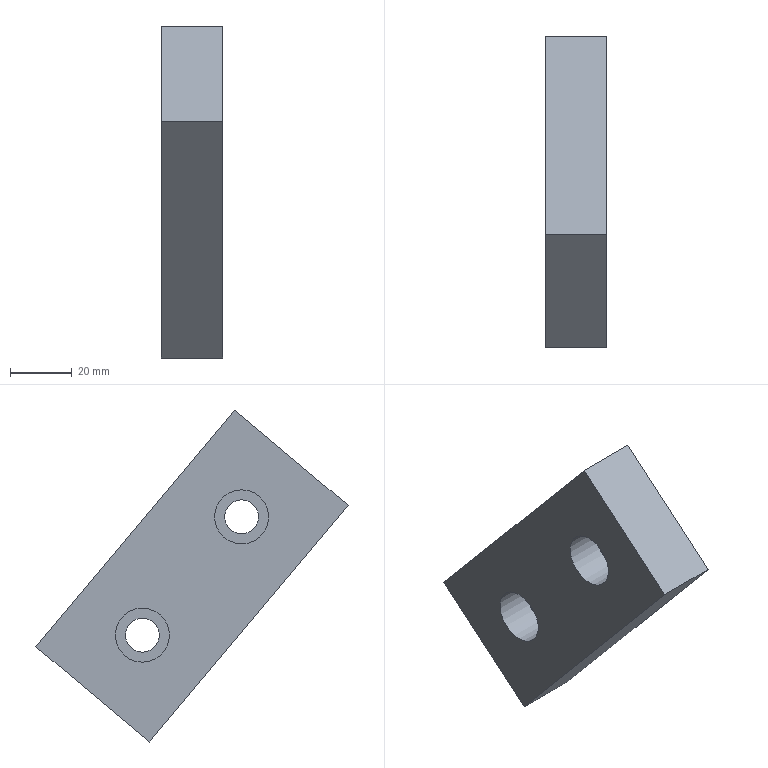Part | NX | features solid 2 | 1 solid | 12 faces | box 20 x 101.049 x 107.458 mm | volume 88707 mm3 | plane 8 | cylinder 4 | commonest cylinder face diameters 11 x2 17.5 x2
STEP:
#1=CARTESIAN_POINT('',(-585.,640.792,26.298));
#2=VERTEX_POINT('',#1);
#3=CARTESIAN_POINT('',(-585.,640.792,17.548));
#4=DIRECTION('',(-1.,0.,0.));
#5=DIRECTION('',(0.,0.,1.));
#6=AXIS2_PLACEMENT_3D('',#3,#4,#5);
#7=CIRCLE('',#6,8.75);
#8=EDGE_CURVE('',#2,#2,#7,.T.);
#9=ORIENTED_EDGE('',*,*,#8,.F.);
#10=EDGE_LOOP('',(#9));
#11=FACE_BOUND('',#10,.T.);
#12=CARTESIAN_POINT('',(-585.,608.652,64.601));
#13=VERTEX_POINT('',#12);
#14=CARTESIAN_POINT('',(-585.,608.652,55.851));
#15=DIRECTION('',(-1.,0.,0.));
#16=DIRECTION('',(0.,0.,1.));
#17=AXIS2_PLACEMENT_3D('',#14,#15,#16);
#18=CIRCLE('',#17,8.75);
#19=EDGE_CURVE('',#13,#13,#18,.T.);
#20=ORIENTED_EDGE('',*,*,#19,.F.);
#21=EDGE_LOOP('',(#20));
#22=FACE_BOUND('',#21,.T.);
#23=CARTESIAN_POINT('',(-585.,610.968,90.429));
#24=VERTEX_POINT('',#23);
#25=CARTESIAN_POINT('',(-585.,574.197,59.575));
#26=VERTEX_POINT('',#25);
#27=CARTESIAN_POINT('',(-585.,612.226,91.485));
#28=DIRECTION('',(0.,0.766,0.6428));
#29=VECTOR('',#28,1000.);
#30=LINE('',#27,#29);
#31=EDGE_CURVE('',#24,#26,#30,.F.);
#32=ORIENTED_EDGE('',*,*,#31,.F.);
#33=CARTESIAN_POINT('',(-585.,675.246,13.824));
#34=VERTEX_POINT('',#33);
#35=CARTESIAN_POINT('',(-585.,675.246,13.824));
#36=DIRECTION('',(0.,-0.6428,0.766));
#37=VECTOR('',#36,1000.);
#38=LINE('',#35,#37);
#39=EDGE_CURVE('',#34,#24,#38,.T.);
#40=ORIENTED_EDGE('',*,*,#39,.F.);
#41=CARTESIAN_POINT('',(-585.,638.476,-17.03));
#42=VERTEX_POINT('',#41);
#43=CARTESIAN_POINT('',(-585.,676.505,14.88));
#44=DIRECTION('',(0.,0.766,0.6428));
#45=VECTOR('',#44,1000.);
#46=LINE('',#43,#45);
#47=EDGE_CURVE('',#34,#42,#46,.F.);
#48=ORIENTED_EDGE('',*,*,#47,.T.);
#49=CARTESIAN_POINT('',(-585.,638.476,-17.03));
#50=DIRECTION('',(0.,0.6428,-0.766));
#51=VECTOR('',#50,1000.);
#52=LINE('',#49,#51);
#53=EDGE_CURVE('',#42,#26,#52,.F.);
#54=ORIENTED_EDGE('',*,*,#53,.T.);
#55=EDGE_LOOP('',(#32,#40,#48,#54));
#56=FACE_BOUND('',#55,.T.);
#57=CARTESIAN_POINT('',(-585.,676.505,14.88));
#58=DIRECTION('',(-1.,0.,0.));
#59=DIRECTION('',(0.,-0.6428,0.766));
#60=AXIS2_PLACEMENT_3D('',#57,#58,#59);
#61=PLANE('',#60);
#62=ADVANCED_FACE('',(#11,#22,#56),#61,.T.);
#63=ORIENTED_EDGE('',*,*,#47,.F.);
#64=CARTESIAN_POINT('',(-565.,675.246,13.824));
#65=VERTEX_POINT('',#64);
#66=CARTESIAN_POINT('',(-585.,675.246,13.824));
#67=DIRECTION('',(1.,0.,0.));
#68=VECTOR('',#67,1000.);
#69=LINE('',#66,#68);
#70=EDGE_CURVE('',#34,#65,#69,.T.);
#71=ORIENTED_EDGE('',*,*,#70,.T.);
#72=CARTESIAN_POINT('',(-565.,638.476,-17.03));
#73=VERTEX_POINT('',#72);
#74=CARTESIAN_POINT('',(-565.,676.505,14.88));
#75=DIRECTION('',(0.,0.766,0.6428));
#76=VECTOR('',#75,1000.);
#77=LINE('',#74,#76);
#78=EDGE_CURVE('',#65,#73,#77,.F.);
#79=ORIENTED_EDGE('',*,*,#78,.T.);
#80=CARTESIAN_POINT('',(-585.,638.476,-17.03));
#81=DIRECTION('',(1.,0.,0.));
#82=VECTOR('',#81,1000.);
#83=LINE('',#80,#82);
#84=EDGE_CURVE('',#42,#73,#83,.T.);
#85=ORIENTED_EDGE('',*,*,#84,.F.);
#86=EDGE_LOOP('',(#63,#71,#79,#85));
#87=FACE_BOUND('',#86,.T.);
#88=CARTESIAN_POINT('',(-585.,676.505,14.88));
#89=DIRECTION('',(0.,-0.6428,0.766));
#90=DIRECTION('',(1.,0.,0.));
#91=AXIS2_PLACEMENT_3D('',#88,#89,#90);
#92=PLANE('',#91);
#93=ADVANCED_FACE('',(#87),#92,.F.);
#94=CARTESIAN_POINT('',(-565.,640.792,12.048));
#95=VERTEX_POINT('',#94);
#96=CARTESIAN_POINT('',(-565.,640.792,17.548));
#97=DIRECTION('',(1.,0.,0.));
#98=DIRECTION('',(0.,0.,-1.));
#99=AXIS2_PLACEMENT_3D('',#96,#97,#98);
#100=CIRCLE('',#99,5.5);
#101=EDGE_CURVE('',#95,#95,#100,.T.);
#102=ORIENTED_EDGE('',*,*,#101,.F.);
#103=EDGE_LOOP('',(#102));
#104=FACE_BOUND('',#103,.T.);
#105=CARTESIAN_POINT('',(-565.,608.652,50.351));
#106=VERTEX_POINT('',#105);
#107=CARTESIAN_POINT('',(-565.,608.652,55.851));
#108=DIRECTION('',(1.,0.,0.));
#109=DIRECTION('',(0.,0.,-1.));
#110=AXIS2_PLACEMENT_3D('',#107,#108,#109);
#111=CIRCLE('',#110,5.5);
#112=EDGE_CURVE('',#106,#106,#111,.T.);
#113=ORIENTED_EDGE('',*,*,#112,.F.);
#114=EDGE_LOOP('',(#113));
#115=FACE_BOUND('',#114,.T.);
#116=ORIENTED_EDGE('',*,*,#78,.F.);
#117=CARTESIAN_POINT('',(-565.,610.968,90.429));
#118=VERTEX_POINT('',#117);
#119=CARTESIAN_POINT('',(-565.,675.246,13.824));
#120=DIRECTION('',(0.,-0.6428,0.766));
#121=VECTOR('',#120,1000.);
#122=LINE('',#119,#121);
#123=EDGE_CURVE('',#65,#118,#122,.T.);
#124=ORIENTED_EDGE('',*,*,#123,.T.);
#125=CARTESIAN_POINT('',(-565.,574.197,59.575));
#126=VERTEX_POINT('',#125);
#127=CARTESIAN_POINT('',(-565.,612.226,91.485));
#128=DIRECTION('',(0.,0.766,0.6428));
#129=VECTOR('',#128,1000.);
#130=LINE('',#127,#129);
#131=EDGE_CURVE('',#118,#126,#130,.F.);
#132=ORIENTED_EDGE('',*,*,#131,.T.);
#133=CARTESIAN_POINT('',(-565.,638.476,-17.03));
#134=DIRECTION('',(0.,-0.6428,0.766));
#135=VECTOR('',#134,1000.);
#136=LINE('',#133,#135);
#137=EDGE_CURVE('',#73,#126,#136,.T.);
#138=ORIENTED_EDGE('',*,*,#137,.F.);
#139=EDGE_LOOP('',(#116,#124,#132,#138));
#140=FACE_BOUND('',#139,.T.);
#141=CARTESIAN_POINT('',(-565.,676.505,14.88));
#142=DIRECTION('',(-1.,0.,0.));
#143=DIRECTION('',(0.,-0.6428,0.766));
#144=AXIS2_PLACEMENT_3D('',#141,#142,#143);
#145=PLANE('',#144);
#146=ADVANCED_FACE('',(#104,#115,#140),#145,.F.);
#147=CARTESIAN_POINT('',(-585.,610.968,90.429));
#148=DIRECTION('',(1.,0.,0.));
#149=VECTOR('',#148,1000.);
#150=LINE('',#147,#149);
#151=EDGE_CURVE('',#24,#118,#150,.T.);
#152=ORIENTED_EDGE('',*,*,#151,.F.);
#153=ORIENTED_EDGE('',*,*,#31,.T.);
#154=CARTESIAN_POINT('',(-585.,574.197,59.575));
#155=DIRECTION('',(-1.,0.,0.));
#156=VECTOR('',#155,1000.);
#157=LINE('',#154,#156);
#158=EDGE_CURVE('',#26,#126,#157,.F.);
#159=ORIENTED_EDGE('',*,*,#158,.T.);
#160=ORIENTED_EDGE('',*,*,#131,.F.);
#161=EDGE_LOOP('',(#152,#153,#159,#160));
#162=FACE_BOUND('',#161,.T.);
#163=CARTESIAN_POINT('',(-585.,612.226,91.485));
#164=DIRECTION('',(0.,-0.6428,0.766));
#165=DIRECTION('',(1.,0.,0.));
#166=AXIS2_PLACEMENT_3D('',#163,#164,#165);
#167=PLANE('',#166);
#168=ADVANCED_FACE('',(#162),#167,.T.);
#169=ORIENTED_EDGE('',*,*,#137,.T.);
#170=ORIENTED_EDGE('',*,*,#158,.F.);
#171=ORIENTED_EDGE('',*,*,#53,.F.);
#172=ORIENTED_EDGE('',*,*,#84,.T.);
#173=EDGE_LOOP('',(#169,#170,#171,#172));
#174=FACE_BOUND('',#173,.T.);
#175=CARTESIAN_POINT('',(-585.,638.476,-17.03));
#176=DIRECTION('',(0.,-0.766,-0.6428));
#177=DIRECTION('',(0.,0.6428,-0.766));
#178=AXIS2_PLACEMENT_3D('',#175,#176,#177);
#179=PLANE('',#178);
#180=ADVANCED_FACE('',(#174),#179,.T.);
#181=ORIENTED_EDGE('',*,*,#123,.F.);
#182=ORIENTED_EDGE('',*,*,#70,.F.);
#183=ORIENTED_EDGE('',*,*,#39,.T.);
#184=ORIENTED_EDGE('',*,*,#151,.T.);
#185=EDGE_LOOP('',(#181,#182,#183,#184));
#186=FACE_BOUND('',#185,.T.);
#187=CARTESIAN_POINT('',(-585.,675.246,13.824));
#188=DIRECTION('',(0.,-0.766,-0.6428));
#189=DIRECTION('',(0.,0.6428,-0.766));
#190=AXIS2_PLACEMENT_3D('',#187,#188,#189);
#191=PLANE('',#190);
#192=ADVANCED_FACE('',(#186),#191,.F.);
#193=CARTESIAN_POINT('',(-573.,608.652,61.351));
#194=VERTEX_POINT('',#193);
#195=CARTESIAN_POINT('',(-573.,608.652,55.851));
#196=DIRECTION('',(-1.,0.,0.));
#197=DIRECTION('',(0.,0.,1.));
#198=AXIS2_PLACEMENT_3D('',#195,#196,#197);
#199=CIRCLE('',#198,5.5);
#200=EDGE_CURVE('',#194,#194,#199,.T.);
#201=ORIENTED_EDGE('',*,*,#200,.T.);
#202=EDGE_LOOP('',(#201));
#203=FACE_BOUND('',#202,.T.);
#204=ORIENTED_EDGE('',*,*,#112,.T.);
#205=EDGE_LOOP('',(#204));
#206=FACE_BOUND('',#205,.T.);
#207=CARTESIAN_POINT('',(-535.,608.652,55.851));
#208=DIRECTION('',(1.,0.,0.));
#209=DIRECTION('',(0.,0.,1.));
#210=AXIS2_PLACEMENT_3D('',#207,#208,#209);
#211=CYLINDRICAL_SURFACE('',#210,5.5);
#212=ADVANCED_FACE('',(#203,#206),#211,.F.);
#213=ORIENTED_EDGE('',*,*,#200,.F.);
#214=EDGE_LOOP('',(#213));
#215=FACE_BOUND('',#214,.T.);
#216=CARTESIAN_POINT('',(-573.,608.652,64.601));
#217=VERTEX_POINT('',#216);
#218=CARTESIAN_POINT('',(-573.,608.652,55.851));
#219=DIRECTION('',(-1.,0.,0.));
#220=DIRECTION('',(0.,0.,1.));
#221=AXIS2_PLACEMENT_3D('',#218,#219,#220);
#222=CIRCLE('',#221,8.75);
#223=EDGE_CURVE('',#217,#217,#222,.T.);
#224=ORIENTED_EDGE('',*,*,#223,.T.);
#225=EDGE_LOOP('',(#224));
#226=FACE_BOUND('',#225,.T.);
#227=CARTESIAN_POINT('',(-573.,609.911,56.907));
#228=DIRECTION('',(1.,0.,0.));
#229=DIRECTION('',(0.,0.,1.));
#230=AXIS2_PLACEMENT_3D('',#227,#228,#229);
#231=PLANE('',#230);
#232=ADVANCED_FACE('',(#215,#226),#231,.F.);
#233=ORIENTED_EDGE('',*,*,#223,.F.);
#234=EDGE_LOOP('',(#233));
#235=FACE_BOUND('',#234,.T.);
#236=ORIENTED_EDGE('',*,*,#19,.T.);
#237=EDGE_LOOP('',(#236));
#238=FACE_BOUND('',#237,.T.);
#239=CARTESIAN_POINT('',(-585.,608.652,55.851));
#240=DIRECTION('',(1.,0.,0.));
#241=DIRECTION('',(0.,0.,1.));
#242=AXIS2_PLACEMENT_3D('',#239,#240,#241);
#243=CYLINDRICAL_SURFACE('',#242,8.75);
#244=ADVANCED_FACE('',(#235,#238),#243,.F.);
#245=CARTESIAN_POINT('',(-573.,640.792,23.048));
#246=VERTEX_POINT('',#245);
#247=CARTESIAN_POINT('',(-573.,640.792,17.548));
#248=DIRECTION('',(-1.,0.,0.));
#249=DIRECTION('',(0.,0.,1.));
#250=AXIS2_PLACEMENT_3D('',#247,#248,#249);
#251=CIRCLE('',#250,5.5);
#252=EDGE_CURVE('',#246,#246,#251,.T.);
#253=ORIENTED_EDGE('',*,*,#252,.T.);
#254=EDGE_LOOP('',(#253));
#255=FACE_BOUND('',#254,.T.);
#256=ORIENTED_EDGE('',*,*,#101,.T.);
#257=EDGE_LOOP('',(#256));
#258=FACE_BOUND('',#257,.T.);
#259=CARTESIAN_POINT('',(-535.,640.792,17.548));
#260=DIRECTION('',(1.,0.,0.));
#261=DIRECTION('',(0.,0.,1.));
#262=AXIS2_PLACEMENT_3D('',#259,#260,#261);
#263=CYLINDRICAL_SURFACE('',#262,5.5);
#264=ADVANCED_FACE('',(#255,#258),#263,.F.);
#265=ORIENTED_EDGE('',*,*,#252,.F.);
#266=EDGE_LOOP('',(#265));
#267=FACE_BOUND('',#266,.T.);
#268=CARTESIAN_POINT('',(-573.,640.792,26.298));
#269=VERTEX_POINT('',#268);
#270=CARTESIAN_POINT('',(-573.,640.792,17.548));
#271=DIRECTION('',(-1.,0.,0.));
#272=DIRECTION('',(0.,0.,1.));
#273=AXIS2_PLACEMENT_3D('',#270,#271,#272);
#274=CIRCLE('',#273,8.75);
#275=EDGE_CURVE('',#269,#269,#274,.T.);
#276=ORIENTED_EDGE('',*,*,#275,.T.);
#277=EDGE_LOOP('',(#276));
#278=FACE_BOUND('',#277,.T.);
#279=CARTESIAN_POINT('',(-573.,642.05,18.604));
#280=DIRECTION('',(1.,0.,0.));
#281=DIRECTION('',(0.,0.,1.));
#282=AXIS2_PLACEMENT_3D('',#279,#280,#281);
#283=PLANE('',#282);
#284=ADVANCED_FACE('',(#267,#278),#283,.F.);
#285=ORIENTED_EDGE('',*,*,#275,.F.);
#286=EDGE_LOOP('',(#285));
#287=FACE_BOUND('',#286,.T.);
#288=ORIENTED_EDGE('',*,*,#8,.T.);
#289=EDGE_LOOP('',(#288));
#290=FACE_BOUND('',#289,.T.);
#291=CARTESIAN_POINT('',(-585.,640.792,17.548));
#292=DIRECTION('',(1.,0.,0.));
#293=DIRECTION('',(0.,0.,1.));
#294=AXIS2_PLACEMENT_3D('',#291,#292,#293);
#295=CYLINDRICAL_SURFACE('',#294,8.75);
#296=ADVANCED_FACE('',(#287,#290),#295,.F.);
#297=CLOSED_SHELL('',(#62,#93,#146,#168,#180,#192,#212,#232,#244,#264,#284,#296));
#298=MANIFOLD_SOLID_BREP('',#297);
#299=(LENGTH_UNIT()NAMED_UNIT(*)SI_UNIT(.MILLI.,.METRE.));
#300=UNCERTAINTY_MEASURE_WITH_UNIT(LENGTH_MEASURE(0.00001),#299,'','');
#301=(NAMED_UNIT(*)PLANE_ANGLE_UNIT()SI_UNIT($,.RADIAN.));
#302=(NAMED_UNIT(*)SI_UNIT($,.STERADIAN.)SOLID_ANGLE_UNIT());
#303=(GEOMETRIC_REPRESENTATION_CONTEXT(3)GLOBAL_UNCERTAINTY_ASSIGNED_CONTEXT((#300))GLOBAL_UNIT_ASSIGNED_CONTEXT((#299,#301,#302))REPRESENTATION_CONTEXT('',''));
#304=ADVANCED_BREP_SHAPE_REPRESENTATION('',(#298),#303);